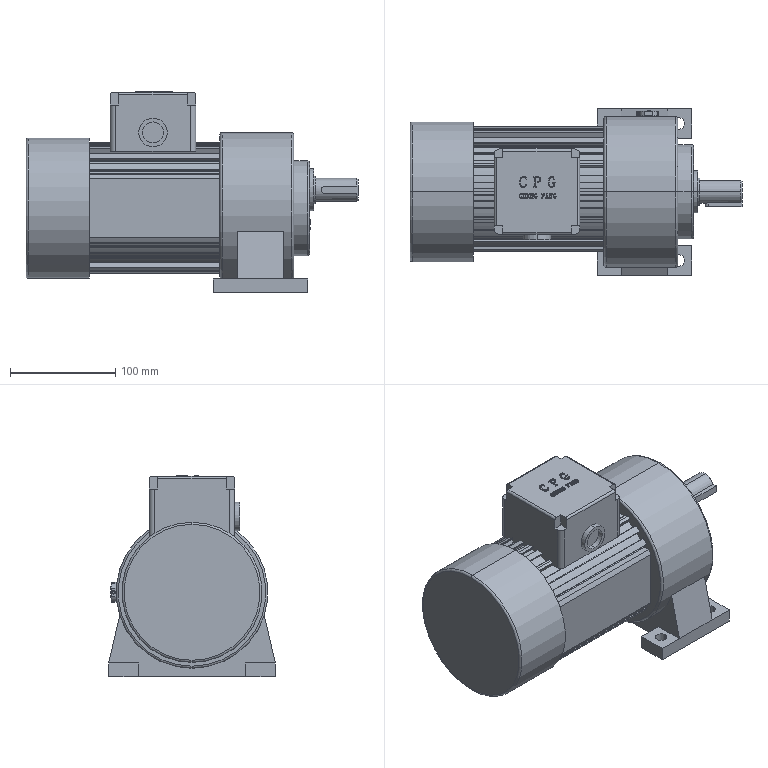Part | SolidWorks | 3 solids | 876 faces | box 315 x 158 x 191 mm | volume 4023427 mm3 | plane 438 | spline 231 | cylinder 196 | torus 8 | cone 3 | commonest cylinder face diameters 1 x43 8 x39 116 x24 124 x16 127 x16 0.3 x8